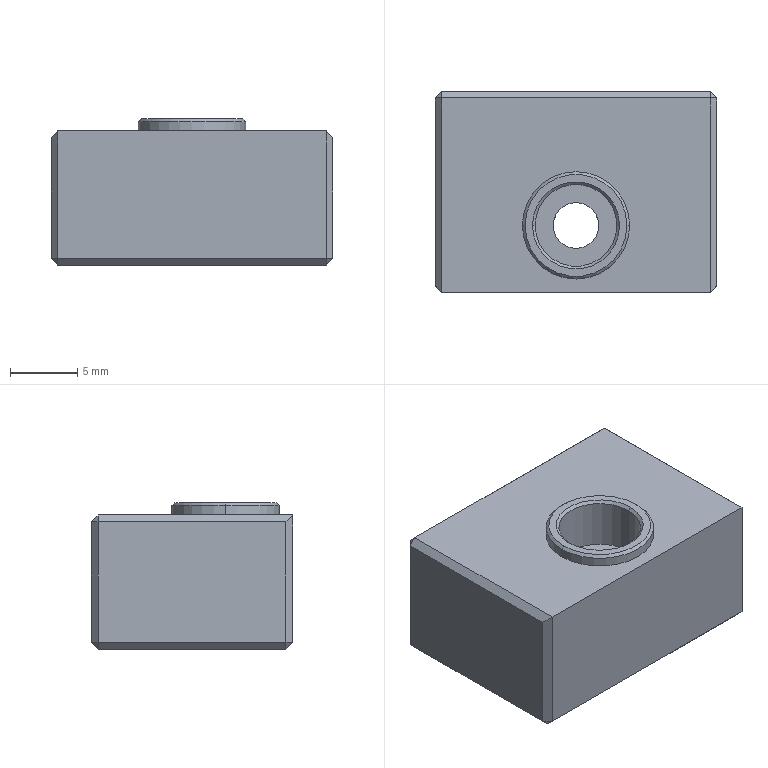Part | STEP file | 10000054265swp000-1 | 1 solid | 46 faces | box 21 x 15 x 10.9 mm | volume 2839 mm3 | plane 26 | cylinder 12 | cone 8 | commonest cylinder face diameters 2.5 x4 3.4 x2 6.1 x2 6.5 x2 8 x2
STEP:
#1=CARTESIAN_POINT('',(3.8,-2.5,5.9));
#2=VERTEX_POINT('',#1);
#3=CARTESIAN_POINT('',(-3.8,-2.5,5.9));
#4=VERTEX_POINT('',#3);
#5=CARTESIAN_POINT('',(0.,-2.5,5.9));
#6=DIRECTION('',(0.,0.,1.));
#7=DIRECTION('',(1.,0.,0.));
#8=AXIS2_PLACEMENT_3D('',#5,#6,#7);
#9=CIRCLE('',#8,3.8);
#10=EDGE_CURVE('',#2,#4,#9,.T.);
#11=ORIENTED_EDGE('',*,*,#10,.F.);
#12=CARTESIAN_POINT('',(4.,-2.5,5.7));
#13=VERTEX_POINT('',#12);
#14=CARTESIAN_POINT('',(3.8,-2.5,5.9));
#15=DIRECTION('',(0.7071,0.,-0.7071));
#16=VECTOR('',#15,1000.);
#17=LINE('',#14,#16);
#18=EDGE_CURVE('',#2,#13,#17,.T.);
#19=ORIENTED_EDGE('',*,*,#18,.T.);
#20=CARTESIAN_POINT('',(-4.,-2.5,5.7));
#21=VERTEX_POINT('',#20);
#22=CARTESIAN_POINT('',(0.,-2.5,5.7));
#23=DIRECTION('',(0.,0.,-1.));
#24=DIRECTION('',(1.,0.,0.));
#25=AXIS2_PLACEMENT_3D('',#22,#23,#24);
#26=CIRCLE('',#25,4.);
#27=EDGE_CURVE('',#21,#13,#26,.T.);
#28=ORIENTED_EDGE('',*,*,#27,.F.);
#29=CARTESIAN_POINT('',(-3.8,-2.5,5.9));
#30=DIRECTION('',(-0.7071,0.,-0.7071));
#31=VECTOR('',#30,1000.);
#32=LINE('',#29,#31);
#33=EDGE_CURVE('',#4,#21,#32,.T.);
#34=ORIENTED_EDGE('',*,*,#33,.F.);
#35=EDGE_LOOP('',(#11,#19,#28,#34));
#36=FACE_OUTER_BOUND('',#35,.T.);
#37=CARTESIAN_POINT('',(0.,-2.5,5.9));
#38=DIRECTION('',(0.,0.,-1.));
#39=DIRECTION('',(-1.,0.,0.));
#40=AXIS2_PLACEMENT_3D('',#37,#38,#39);
#41=CONICAL_SURFACE('',#40,3.8,0.7854);
#42=ADVANCED_FACE('',(#36),#41,.T.);
#43=CARTESIAN_POINT('',(-3.05,-2.5,5.7));
#44=VERTEX_POINT('',#43);
#45=CARTESIAN_POINT('',(3.05,-2.5,5.7));
#46=VERTEX_POINT('',#45);
#47=CARTESIAN_POINT('',(0.,-2.5,5.7));
#48=DIRECTION('',(0.,0.,1.));
#49=DIRECTION('',(1.,0.,0.));
#50=AXIS2_PLACEMENT_3D('',#47,#48,#49);
#51=CIRCLE('',#50,3.05);
#52=EDGE_CURVE('',#44,#46,#51,.T.);
#53=ORIENTED_EDGE('',*,*,#52,.F.);
#54=CARTESIAN_POINT('',(-3.25,-2.5,5.9));
#55=VERTEX_POINT('',#54);
#56=CARTESIAN_POINT('',(-3.05,-2.5,5.7));
#57=DIRECTION('',(-0.7071,0.,0.7071));
#58=VECTOR('',#57,1000.);
#59=LINE('',#56,#58);
#60=EDGE_CURVE('',#44,#55,#59,.T.);
#61=ORIENTED_EDGE('',*,*,#60,.T.);
#62=CARTESIAN_POINT('',(3.25,-2.5,5.9));
#63=VERTEX_POINT('',#62);
#64=CARTESIAN_POINT('',(0.,-2.5,5.9));
#65=DIRECTION('',(0.,0.,-1.));
#66=DIRECTION('',(1.,0.,0.));
#67=AXIS2_PLACEMENT_3D('',#64,#65,#66);
#68=CIRCLE('',#67,3.25);
#69=EDGE_CURVE('',#63,#55,#68,.T.);
#70=ORIENTED_EDGE('',*,*,#69,.F.);
#71=CARTESIAN_POINT('',(3.05,-2.5,5.7));
#72=DIRECTION('',(0.7071,0.,0.7071));
#73=VECTOR('',#72,1000.);
#74=LINE('',#71,#73);
#75=EDGE_CURVE('',#46,#63,#74,.T.);
#76=ORIENTED_EDGE('',*,*,#75,.F.);
#77=EDGE_LOOP('',(#53,#61,#70,#76));
#78=FACE_OUTER_BOUND('',#77,.T.);
#79=CARTESIAN_POINT('',(0.,-2.5,5.7));
#80=DIRECTION('',(0.,0.,1.));
#81=DIRECTION('',(1.,0.,0.));
#82=AXIS2_PLACEMENT_3D('',#79,#80,#81);
#83=CONICAL_SURFACE('',#82,3.05,0.7854);
#84=ADVANCED_FACE('',(#78),#83,.F.);
#85=CARTESIAN_POINT('',(3.25,-2.5,-1.6));
#86=VERTEX_POINT('',#85);
#87=CARTESIAN_POINT('',(-3.25,-2.5,-1.6));
#88=VERTEX_POINT('',#87);
#89=CARTESIAN_POINT('',(0.,-2.5,-1.6));
#90=DIRECTION('',(0.,0.,-1.));
#91=DIRECTION('',(-1.,0.,0.));
#92=AXIS2_PLACEMENT_3D('',#89,#90,#91);
#93=CIRCLE('',#92,3.25);
#94=EDGE_CURVE('',#86,#88,#93,.T.);
#95=ORIENTED_EDGE('',*,*,#94,.F.);
#96=CARTESIAN_POINT('',(3.25,-2.5,-5.));
#97=VERTEX_POINT('',#96);
#98=CARTESIAN_POINT('',(3.25,-2.5,-5.));
#99=DIRECTION('',(0.,0.,-1.));
#100=VECTOR('',#99,1000.);
#101=LINE('',#98,#100);
#102=EDGE_CURVE('',#86,#97,#101,.T.);
#103=ORIENTED_EDGE('',*,*,#102,.T.);
#104=CARTESIAN_POINT('',(-3.25,-2.5,-5.));
#105=VERTEX_POINT('',#104);
#106=CARTESIAN_POINT('',(0.,-2.5,-5.));
#107=DIRECTION('',(0.,0.,-1.));
#108=DIRECTION('',(-1.,0.,0.));
#109=AXIS2_PLACEMENT_3D('',#106,#107,#108);
#110=CIRCLE('',#109,3.25);
#111=EDGE_CURVE('',#97,#105,#110,.T.);
#112=ORIENTED_EDGE('',*,*,#111,.T.);
#113=CARTESIAN_POINT('',(-3.25,-2.5,-5.));
#114=DIRECTION('',(0.,0.,-1.));
#115=VECTOR('',#114,1000.);
#116=LINE('',#113,#115);
#117=EDGE_CURVE('',#88,#105,#116,.T.);
#118=ORIENTED_EDGE('',*,*,#117,.F.);
#119=EDGE_LOOP('',(#95,#103,#112,#118));
#120=FACE_OUTER_BOUND('',#119,.T.);
#121=CARTESIAN_POINT('',(0.,-2.5,-5.));
#122=DIRECTION('',(0.,0.,-1.));
#123=DIRECTION('',(-1.,0.,0.));
#124=AXIS2_PLACEMENT_3D('',#121,#122,#123);
#125=CYLINDRICAL_SURFACE('',#124,3.25);
#126=ADVANCED_FACE('',(#120),#125,.F.);
#127=CARTESIAN_POINT('',(1.7,-2.5,2.));
#128=VERTEX_POINT('',#127);
#129=CARTESIAN_POINT('',(-1.7,-2.5,2.));
#130=VERTEX_POINT('',#129);
#131=CARTESIAN_POINT('',(0.,-2.5,2.));
#132=DIRECTION('',(0.,0.,-1.));
#133=DIRECTION('',(-1.,0.,0.));
#134=AXIS2_PLACEMENT_3D('',#131,#132,#133);
#135=CIRCLE('',#134,1.7);
#136=EDGE_CURVE('',#128,#130,#135,.T.);
#137=ORIENTED_EDGE('',*,*,#136,.F.);
#138=CARTESIAN_POINT('',(1.7,-2.5,-1.6));
#139=VERTEX_POINT('',#138);
#140=CARTESIAN_POINT('',(1.7,-2.5,-5.));
#141=DIRECTION('',(0.,0.,-1.));
#142=VECTOR('',#141,1000.);
#143=LINE('',#140,#142);
#144=EDGE_CURVE('',#128,#139,#143,.T.);
#145=ORIENTED_EDGE('',*,*,#144,.T.);
#146=CARTESIAN_POINT('',(-1.7,-2.5,-1.6));
#147=VERTEX_POINT('',#146);
#148=CARTESIAN_POINT('',(0.,-2.5,-1.6));
#149=DIRECTION('',(0.,0.,-1.));
#150=DIRECTION('',(-1.,0.,0.));
#151=AXIS2_PLACEMENT_3D('',#148,#149,#150);
#152=CIRCLE('',#151,1.7);
#153=EDGE_CURVE('',#139,#147,#152,.T.);
#154=ORIENTED_EDGE('',*,*,#153,.T.);
#155=CARTESIAN_POINT('',(-1.7,-2.5,-5.));
#156=DIRECTION('',(0.,0.,-1.));
#157=VECTOR('',#156,1000.);
#158=LINE('',#155,#157);
#159=EDGE_CURVE('',#130,#147,#158,.T.);
#160=ORIENTED_EDGE('',*,*,#159,.F.);
#161=EDGE_LOOP('',(#137,#145,#154,#160));
#162=FACE_OUTER_BOUND('',#161,.T.);
#163=CARTESIAN_POINT('',(0.,-2.5,-5.));
#164=DIRECTION('',(0.,0.,-1.));
#165=DIRECTION('',(-1.,0.,0.));
#166=AXIS2_PLACEMENT_3D('',#163,#164,#165);
#167=CYLINDRICAL_SURFACE('',#166,1.7);
#168=ADVANCED_FACE('',(#162),#167,.F.);
#169=CARTESIAN_POINT('',(-3.05,-2.5,2.));
#170=VERTEX_POINT('',#169);
#171=CARTESIAN_POINT('',(3.05,-2.5,2.));
#172=VERTEX_POINT('',#171);
#173=CARTESIAN_POINT('',(0.,-2.5,2.));
#174=DIRECTION('',(0.,0.,1.));
#175=DIRECTION('',(1.,0.,0.));
#176=AXIS2_PLACEMENT_3D('',#173,#174,#175);
#177=CIRCLE('',#176,3.05);
#178=EDGE_CURVE('',#170,#172,#177,.T.);
#179=ORIENTED_EDGE('',*,*,#178,.F.);
#180=CARTESIAN_POINT('',(-3.05,-2.5,5.));
#181=DIRECTION('',(0.,0.,1.));
#182=VECTOR('',#181,1000.);
#183=LINE('',#180,#182);
#184=EDGE_CURVE('',#170,#44,#183,.T.);
#185=ORIENTED_EDGE('',*,*,#184,.T.);
#186=ORIENTED_EDGE('',*,*,#52,.T.);
#187=CARTESIAN_POINT('',(3.05,-2.5,5.));
#188=DIRECTION('',(0.,0.,1.));
#189=VECTOR('',#188,1000.);
#190=LINE('',#187,#189);
#191=EDGE_CURVE('',#172,#46,#190,.T.);
#192=ORIENTED_EDGE('',*,*,#191,.F.);
#193=EDGE_LOOP('',(#179,#185,#186,#192));
#194=FACE_OUTER_BOUND('',#193,.T.);
#195=CARTESIAN_POINT('',(0.,-2.5,5.));
#196=DIRECTION('',(0.,0.,1.));
#197=DIRECTION('',(1.,0.,0.));
#198=AXIS2_PLACEMENT_3D('',#195,#196,#197);
#199=CYLINDRICAL_SURFACE('',#198,3.05);
#200=ADVANCED_FACE('',(#194),#199,.F.);
#201=ORIENTED_EDGE('',*,*,#27,.T.);
#202=CARTESIAN_POINT('',(4.,-2.5,5.));
#203=VERTEX_POINT('',#202);
#204=CARTESIAN_POINT('',(4.,-2.5,5.9));
#205=DIRECTION('',(0.,0.,-1.));
#206=VECTOR('',#205,1000.);
#207=LINE('',#204,#206);
#208=EDGE_CURVE('',#13,#203,#207,.T.);
#209=ORIENTED_EDGE('',*,*,#208,.T.);
#210=CARTESIAN_POINT('',(-4.,-2.5,5.));
#211=VERTEX_POINT('',#210);
#212=CARTESIAN_POINT('',(0.,-2.5,5.));
#213=DIRECTION('',(0.,0.,1.));
#214=DIRECTION('',(1.,0.,0.));
#215=AXIS2_PLACEMENT_3D('',#212,#213,#214);
#216=CIRCLE('',#215,4.);
#217=EDGE_CURVE('',#203,#211,#216,.T.);
#218=ORIENTED_EDGE('',*,*,#217,.T.);
#219=CARTESIAN_POINT('',(-4.,-2.5,5.9));
#220=DIRECTION('',(0.,0.,-1.));
#221=VECTOR('',#220,1000.);
#222=LINE('',#219,#221);
#223=EDGE_CURVE('',#21,#211,#222,.T.);
#224=ORIENTED_EDGE('',*,*,#223,.F.);
#225=EDGE_LOOP('',(#201,#209,#218,#224));
#226=FACE_OUTER_BOUND('',#225,.T.);
#227=CARTESIAN_POINT('',(0.,-2.5,5.9));
#228=DIRECTION('',(0.,0.,-1.));
#229=DIRECTION('',(-1.,0.,0.));
#230=AXIS2_PLACEMENT_3D('',#227,#228,#229);
#231=CYLINDRICAL_SURFACE('',#230,4.);
#232=ADVANCED_FACE('',(#226),#231,.T.);
#233=CARTESIAN_POINT('',(-5.5,0.,-1.25));
#234=VERTEX_POINT('',#233);
#235=CARTESIAN_POINT('',(-5.5,0.,1.25));
#236=VERTEX_POINT('',#235);
#237=CARTESIAN_POINT('',(-5.5,0.,0.));
#238=DIRECTION('',(0.,1.,0.));
#239=DIRECTION('',(0.,0.,1.));
#240=AXIS2_PLACEMENT_3D('',#237,#238,#239);
#241=CIRCLE('',#240,1.25);
#242=EDGE_CURVE('',#234,#236,#241,.T.);
#243=ORIENTED_EDGE('',*,*,#242,.F.);
#244=CARTESIAN_POINT('',(-5.5,7.5,-1.25));
#245=VERTEX_POINT('',#244);
#246=CARTESIAN_POINT('',(-5.5,7.5,-1.25));
#247=DIRECTION('',(0.,1.,0.));
#248=VECTOR('',#247,1000.);
#249=LINE('',#246,#248);
#250=EDGE_CURVE('',#234,#245,#249,.T.);
#251=ORIENTED_EDGE('',*,*,#250,.T.);
#252=CARTESIAN_POINT('',(-5.5,7.5,1.25));
#253=VERTEX_POINT('',#252);
#254=CARTESIAN_POINT('',(-5.5,7.5,0.));
#255=DIRECTION('',(0.,1.,0.));
#256=DIRECTION('',(0.,0.,1.));
#257=AXIS2_PLACEMENT_3D('',#254,#255,#256);
#258=CIRCLE('',#257,1.25);
#259=EDGE_CURVE('',#245,#253,#258,.T.);
#260=ORIENTED_EDGE('',*,*,#259,.T.);
#261=CARTESIAN_POINT('',(-5.5,7.5,1.25));
#262=DIRECTION('',(0.,1.,0.));
#263=VECTOR('',#262,1000.);
#264=LINE('',#261,#263);
#265=EDGE_CURVE('',#236,#253,#264,.T.);
#266=ORIENTED_EDGE('',*,*,#265,.F.);
#267=EDGE_LOOP('',(#243,#251,#260,#266));
#268=FACE_OUTER_BOUND('',#267,.T.);
#269=CARTESIAN_POINT('',(-5.5,7.5,0.));
#270=DIRECTION('',(0.,1.,0.));
#271=DIRECTION('',(0.,0.,1.));
#272=AXIS2_PLACEMENT_3D('',#269,#270,#271);
#273=CYLINDRICAL_SURFACE('',#272,1.25);
#274=ADVANCED_FACE('',(#268),#273,.F.);
#275=CARTESIAN_POINT('',(-5.5,-0.7511,0.));
#276=VERTEX_POINT('',#275);
#277=CARTESIAN_POINT('',(-5.5,0.,1.25));
#278=DIRECTION('',(0.,0.515,0.8572));
#279=VECTOR('',#278,1000.);
#280=LINE('',#277,#279);
#281=EDGE_CURVE('',#276,#236,#280,.T.);
#282=ORIENTED_EDGE('',*,*,#281,.F.);
#283=CARTESIAN_POINT('',(-5.5,0.,-1.25));
#284=DIRECTION('',(0.,0.515,-0.8572));
#285=VECTOR('',#284,1000.);
#286=LINE('',#283,#285);
#287=EDGE_CURVE('',#276,#234,#286,.T.);
#288=ORIENTED_EDGE('',*,*,#287,.T.);
#289=ORIENTED_EDGE('',*,*,#242,.T.);
#290=EDGE_LOOP('',(#282,#288,#289));
#291=FACE_OUTER_BOUND('',#290,.T.);
#292=CARTESIAN_POINT('',(-5.5,0.,0.));
#293=DIRECTION('',(0.,1.,0.));
#294=DIRECTION('',(0.,0.,1.));
#295=AXIS2_PLACEMENT_3D('',#292,#293,#294);
#296=CONICAL_SURFACE('',#295,1.25,1.03);
#297=ADVANCED_FACE('',(#291),#296,.F.);
#298=CARTESIAN_POINT('',(5.5,0.,-1.25));
#299=VERTEX_POINT('',#298);
#300=CARTESIAN_POINT('',(5.5,0.,1.25));
#301=VERTEX_POINT('',#300);
#302=CARTESIAN_POINT('',(5.5,0.,0.));
#303=DIRECTION('',(0.,1.,0.));
#304=DIRECTION('',(0.,0.,1.));
#305=AXIS2_PLACEMENT_3D('',#302,#303,#304);
#306=CIRCLE('',#305,1.25);
#307=EDGE_CURVE('',#299,#301,#306,.T.);
#308=ORIENTED_EDGE('',*,*,#307,.F.);
#309=CARTESIAN_POINT('',(5.5,7.5,-1.25));
#310=VERTEX_POINT('',#309);
#311=CARTESIAN_POINT('',(5.5,7.5,-1.25));
#312=DIRECTION('',(0.,1.,0.));
#313=VECTOR('',#312,1000.);
#314=LINE('',#311,#313);
#315=EDGE_CURVE('',#299,#310,#314,.T.);
#316=ORIENTED_EDGE('',*,*,#315,.T.);
#317=CARTESIAN_POINT('',(5.5,7.5,1.25));
#318=VERTEX_POINT('',#317);
#319=CARTESIAN_POINT('',(5.5,7.5,0.));
#320=DIRECTION('',(0.,1.,0.));
#321=DIRECTION('',(0.,0.,1.));
#322=AXIS2_PLACEMENT_3D('',#319,#320,#321);
#323=CIRCLE('',#322,1.25);
#324=EDGE_CURVE('',#310,#318,#323,.T.);
#325=ORIENTED_EDGE('',*,*,#324,.T.);
#326=CARTESIAN_POINT('',(5.5,7.5,1.25));
#327=DIRECTION('',(0.,1.,0.));
#328=VECTOR('',#327,1000.);
#329=LINE('',#326,#328);
#330=EDGE_CURVE('',#301,#318,#329,.T.);
#331=ORIENTED_EDGE('',*,*,#330,.F.);
#332=EDGE_LOOP('',(#308,#316,#325,#331));
#333=FACE_OUTER_BOUND('',#332,.T.);
#334=CARTESIAN_POINT('',(5.5,7.5,0.));
#335=DIRECTION('',(0.,1.,0.));
#336=DIRECTION('',(0.,0.,1.));
#337=AXIS2_PLACEMENT_3D('',#334,#335,#336);
#338=CYLINDRICAL_SURFACE('',#337,1.25);
#339=ADVANCED_FACE('',(#333),#338,.F.);
#340=CARTESIAN_POINT('',(5.5,-0.7511,0.));
#341=VERTEX_POINT('',#340);
#342=CARTESIAN_POINT('',(5.5,0.,1.25));
#343=DIRECTION('',(0.,0.515,0.8572));
#344=VECTOR('',#343,1000.);
#345=LINE('',#342,#344);
#346=EDGE_CURVE('',#341,#301,#345,.T.);
#347=ORIENTED_EDGE('',*,*,#346,.F.);
#348=CARTESIAN_POINT('',(5.5,0.,-1.25));
#349=DIRECTION('',(0.,0.515,-0.8572));
#350=VECTOR('',#349,1000.);
#351=LINE('',#348,#350);
#352=EDGE_CURVE('',#341,#299,#351,.T.);
#353=ORIENTED_EDGE('',*,*,#352,.T.);
#354=ORIENTED_EDGE('',*,*,#307,.T.);
#355=EDGE_LOOP('',(#347,#353,#354));
#356=FACE_OUTER_BOUND('',#355,.T.);
#357=CARTESIAN_POINT('',(5.5,0.,0.));
#358=DIRECTION('',(0.,1.,0.));
#359=DIRECTION('',(0.,0.,1.));
#360=AXIS2_PLACEMENT_3D('',#357,#358,#359);
#361=CONICAL_SURFACE('',#360,1.25,1.03);
#362=ADVANCED_FACE('',(#356),#361,.F.);
#363=CARTESIAN_POINT('',(-10.,-7.5,5.));
#364=VERTEX_POINT('',#363);
#365=CARTESIAN_POINT('',(10.,-7.5,5.));
#366=VERTEX_POINT('',#365);
#367=CARTESIAN_POINT('',(-10.5,-7.5,5.));
#368=DIRECTION('',(1.,0.,0.));
#369=VECTOR('',#368,1000.);
#370=LINE('',#367,#369);
#371=EDGE_CURVE('',#364,#366,#370,.T.);
#372=ORIENTED_EDGE('',*,*,#371,.T.);
#373=CARTESIAN_POINT('',(10.,7.,5.));
#374=VERTEX_POINT('',#373);
#375=CARTESIAN_POINT('',(10.,7.5,5.));
#376=DIRECTION('',(0.,1.,0.));
#377=VECTOR('',#376,1000.);
#378=LINE('',#375,#377);
#379=EDGE_CURVE('',#366,#374,#378,.T.);
#380=ORIENTED_EDGE('',*,*,#379,.T.);
#381=CARTESIAN_POINT('',(-10.,7.,5.));
#382=VERTEX_POINT('',#381);
#383=CARTESIAN_POINT('',(-10.5,7.,5.));
#384=DIRECTION('',(-1.,0.,0.));
#385=VECTOR('',#384,1000.);
#386=LINE('',#383,#385);
#387=EDGE_CURVE('',#374,#382,#386,.T.);
#388=ORIENTED_EDGE('',*,*,#387,.T.);
#389=CARTESIAN_POINT('',(-10.,-7.5,5.));
#390=DIRECTION('',(0.,-1.,0.));
#391=VECTOR('',#390,1000.);
#392=LINE('',#389,#391);
#393=EDGE_CURVE('',#382,#364,#392,.T.);
#394=ORIENTED_EDGE('',*,*,#393,.T.);
#395=EDGE_LOOP('',(#372,#380,#388,#394));
#396=FACE_OUTER_BOUND('',#395,.T.);
#397=CARTESIAN_POINT('',(0.,-2.5,5.));
#398=DIRECTION('',(0.,0.,1.));
#399=DIRECTION('',(1.,0.,0.));
#400=AXIS2_PLACEMENT_3D('',#397,#398,#399);
#401=CIRCLE('',#400,4.);
#402=EDGE_CURVE('',#211,#203,#401,.T.);
#403=ORIENTED_EDGE('',*,*,#402,.F.);
#404=ORIENTED_EDGE('',*,*,#217,.F.);
#405=EDGE_LOOP('',(#403,#404));
#406=FACE_BOUND('',#405,.T.);
#407=CARTESIAN_POINT('',(0.,0.,5.));
#408=DIRECTION('',(0.,0.,1.));
#409=DIRECTION('',(1.,0.,0.));
#410=AXIS2_PLACEMENT_3D('',#407,#408,#409);
#411=PLANE('',#410);
#412=ADVANCED_FACE('',(#396,#406),#411,.T.);
#413=CARTESIAN_POINT('',(10.5,7.,-4.5));
#414=VERTEX_POINT('',#413);
#415=CARTESIAN_POINT('',(10.5,7.,4.5));
#416=VERTEX_POINT('',#415);
#417=CARTESIAN_POINT('',(10.5,7.,5.));
#418=DIRECTION('',(0.,0.,1.));
#419=VECTOR('',#418,1000.);
#420=LINE('',#417,#419);
#421=EDGE_CURVE('',#414,#416,#420,.T.);
#422=ORIENTED_EDGE('',*,*,#421,.T.);
#423=CARTESIAN_POINT('',(10.5,-7.,4.5));
#424=VERTEX_POINT('',#423);
#425=CARTESIAN_POINT('',(10.5,-7.5,4.5));
#426=DIRECTION('',(0.,-1.,0.));
#427=VECTOR('',#426,1000.);
#428=LINE('',#425,#427);
#429=EDGE_CURVE('',#416,#424,#428,.T.);
#430=ORIENTED_EDGE('',*,*,#429,.T.);
#431=CARTESIAN_POINT('',(10.5,-7.,-4.5));
#432=VERTEX_POINT('',#431);
#433=CARTESIAN_POINT('',(10.5,-7.,5.));
#434=DIRECTION('',(0.,0.,-1.));
#435=VECTOR('',#434,1000.);
#436=LINE('',#433,#435);
#437=EDGE_CURVE('',#424,#432,#436,.T.);
#438=ORIENTED_EDGE('',*,*,#437,.T.);
#439=CARTESIAN_POINT('',(10.5,7.5,-4.5));
#440=DIRECTION('',(0.,1.,0.));
#441=VECTOR('',#440,1000.);
#442=LINE('',#439,#441);
#443=EDGE_CURVE('',#432,#414,#442,.T.);
#444=ORIENTED_EDGE('',*,*,#443,.T.);
#445=EDGE_LOOP('',(#422,#430,#438,#444));
#446=FACE_OUTER_BOUND('',#445,.T.);
#447=CARTESIAN_POINT('',(10.5,7.5,5.));
#448=DIRECTION('',(-1.,0.,0.));
#449=DIRECTION('',(0.,0.,1.));
#450=AXIS2_PLACEMENT_3D('',#447,#448,#449);
#451=PLANE('',#450);
#452=ADVANCED_FACE('',(#446),#451,.F.);
#453=CARTESIAN_POINT('',(-10.,7.5,-4.5));
#454=VERTEX_POINT('',#453);
#455=CARTESIAN_POINT('',(-10.,7.5,4.5));
#456=VERTEX_POINT('',#455);
#457=CARTESIAN_POINT('',(-10.,7.5,5.));
#458=DIRECTION('',(0.,0.,1.));
#459=VECTOR('',#458,1000.);
#460=LINE('',#457,#459);
#461=EDGE_CURVE('',#454,#456,#460,.T.);
#462=ORIENTED_EDGE('',*,*,#461,.T.);
#463=CARTESIAN_POINT('',(10.,7.5,4.5));
#464=VERTEX_POINT('',#463);
#465=CARTESIAN_POINT('',(10.5,7.5,4.5));
#466=DIRECTION('',(1.,0.,0.));
#467=VECTOR('',#466,1000.);
#468=LINE('',#465,#467);
#469=EDGE_CURVE('',#456,#464,#468,.T.);
#470=ORIENTED_EDGE('',*,*,#469,.T.);
#471=CARTESIAN_POINT('',(10.,7.5,-4.5));
#472=VERTEX_POINT('',#471);
#473=CARTESIAN_POINT('',(10.,7.5,5.));
#474=DIRECTION('',(0.,0.,-1.));
#475=VECTOR('',#474,1000.);
#476=LINE('',#473,#475);
#477=EDGE_CURVE('',#464,#472,#476,.T.);
#478=ORIENTED_EDGE('',*,*,#477,.T.);
#479=CARTESIAN_POINT('',(-10.5,7.5,-4.5));
#480=DIRECTION('',(-1.,0.,0.));
#481=VECTOR('',#480,1000.);
#482=LINE('',#479,#481);
#483=EDGE_CURVE('',#472,#454,#482,.T.);
#484=ORIENTED_EDGE('',*,*,#483,.T.);
#485=EDGE_LOOP('',(#462,#470,#478,#484));
#486=FACE_OUTER_BOUND('',#485,.T.);
#487=CARTESIAN_POINT('',(-5.5,7.5,0.));
#488=DIRECTION('',(0.,1.,0.));
#489=DIRECTION('',(0.,0.,1.));
#490=AXIS2_PLACEMENT_3D('',#487,#488,#489);
#491=CIRCLE('',#490,1.25);
#492=EDGE_CURVE('',#253,#245,#491,.T.);
#493=ORIENTED_EDGE('',*,*,#492,.F.);
#494=ORIENTED_EDGE('',*,*,#259,.F.);
#495=EDGE_LOOP('',(#493,#494));
#496=FACE_BOUND('',#495,.T.);
#497=CARTESIAN_POINT('',(5.5,7.5,0.));
#498=DIRECTION('',(0.,1.,0.));
#499=DIRECTION('',(0.,0.,1.));
#500=AXIS2_PLACEMENT_3D('',#497,#498,#499);
#501=CIRCLE('',#500,1.25);
#502=EDGE_CURVE('',#318,#310,#501,.T.);
#503=ORIENTED_EDGE('',*,*,#502,.F.);
#504=ORIENTED_EDGE('',*,*,#324,.F.);
#505=EDGE_LOOP('',(#503,#504));
#506=FACE_BOUND('',#505,.T.);
#507=CARTESIAN_POINT('',(-10.5,7.5,5.));
#508=DIRECTION('',(0.,-1.,0.));
#509=DIRECTION('',(0.,0.,-1.));
#510=AXIS2_PLACEMENT_3D('',#507,#508,#509);
#511=PLANE('',#510);
#512=ADVANCED_FACE('',(#486,#496,#506),#511,.F.);
#513=CARTESIAN_POINT('',(-10.5,-7.,-4.5));
#514=VERTEX_POINT('',#513);
#515=CARTESIAN_POINT('',(-10.5,-7.,4.5));
#516=VERTEX_POINT('',#515);
#517=CARTESIAN_POINT('',(-10.5,-7.,5.));
#518=DIRECTION('',(0.,0.,1.));
#519=VECTOR('',#518,1000.);
#520=LINE('',#517,#519);
#521=EDGE_CURVE('',#514,#516,#520,.T.);
#522=ORIENTED_EDGE('',*,*,#521,.T.);
#523=CARTESIAN_POINT('',(-10.5,7.,4.5));
#524=VERTEX_POINT('',#523);
#525=CARTESIAN_POINT('',(-10.5,7.5,4.5));
#526=DIRECTION('',(0.,1.,0.));
#527=VECTOR('',#526,1000.);
#528=LINE('',#525,#527);
#529=EDGE_CURVE('',#516,#524,#528,.T.);
#530=ORIENTED_EDGE('',*,*,#529,.T.);
#531=CARTESIAN_POINT('',(-10.5,7.,-4.5));
#532=VERTEX_POINT('',#531);
#533=CARTESIAN_POINT('',(-10.5,7.,5.));
#534=DIRECTION('',(0.,0.,-1.));
#535=VECTOR('',#534,1000.);
#536=LINE('',#533,#535);
#537=EDGE_CURVE('',#524,#532,#536,.T.);
#538=ORIENTED_EDGE('',*,*,#537,.T.);
#539=CARTESIAN_POINT('',(-10.5,7.5,-4.5));
#540=DIRECTION('',(0.,-1.,0.));
#541=VECTOR('',#540,1000.);
#542=LINE('',#539,#541);
#543=EDGE_CURVE('',#532,#514,#542,.T.);
#544=ORIENTED_EDGE('',*,*,#543,.T.);
#545=EDGE_LOOP('',(#522,#530,#538,#544));
#546=FACE_OUTER_BOUND('',#545,.T.);
#547=CARTESIAN_POINT('',(-10.5,7.5,5.));
#548=DIRECTION('',(1.,0.,0.));
#549=DIRECTION('',(0.,0.,-1.));
#550=AXIS2_PLACEMENT_3D('',#547,#548,#549);
#551=PLANE('',#550);
#552=ADVANCED_FACE('',(#546),#551,.F.);
#553=ORIENTED_EDGE('',*,*,#371,.F.);
#554=CARTESIAN_POINT('',(-10.,-7.5,-4.5));
#555=VERTEX_POINT('',#554);
#556=CARTESIAN_POINT('',(-10.,-7.5,5.));
#557=DIRECTION('',(0.,0.,-1.));
#558=VECTOR('',#557,1000.);
#559=LINE('',#556,#558);
#560=EDGE_CURVE('',#364,#555,#559,.T.);
#561=ORIENTED_EDGE('',*,*,#560,.T.);
#562=CARTESIAN_POINT('',(10.,-7.5,-4.5));
#563=VERTEX_POINT('',#562);
#564=CARTESIAN_POINT('',(-10.5,-7.5,-4.5));
#565=DIRECTION('',(1.,0.,0.));
#566=VECTOR('',#565,1000.);
#567=LINE('',#564,#566);
#568=EDGE_CURVE('',#555,#563,#567,.T.);
#569=ORIENTED_EDGE('',*,*,#568,.T.);
#570=CARTESIAN_POINT('',(10.,-7.5,5.));
#571=DIRECTION('',(0.,0.,1.));
#572=VECTOR('',#571,1000.);
#573=LINE('',#570,#572);
#574=EDGE_CURVE('',#563,#366,#573,.T.);
#575=ORIENTED_EDGE('',*,*,#574,.T.);
#576=EDGE_LOOP('',(#553,#561,#569,#575));
#577=FACE_OUTER_BOUND('',#576,.T.);
#578=CARTESIAN_POINT('',(-10.5,-7.5,5.));
#579=DIRECTION('',(0.,1.,0.));
#580=DIRECTION('',(0.,0.,1.));
#581=AXIS2_PLACEMENT_3D('',#578,#579,#580);
#582=PLANE('',#581);
#583=ADVANCED_FACE('',(#577),#582,.F.);
#584=CARTESIAN_POINT('',(10.,7.,-5.));
#585=VERTEX_POINT('',#584);
#586=CARTESIAN_POINT('',(10.,-7.,-5.));
#587=VERTEX_POINT('',#586);
#588=CARTESIAN_POINT('',(10.,0.,-5.));
#589=DIRECTION('',(0.,-1.,0.));
#590=VECTOR('',#589,1000.);
#591=LINE('',#588,#590);
#592=EDGE_CURVE('',#585,#587,#591,.T.);
#593=ORIENTED_EDGE('',*,*,#592,.T.);
#594=CARTESIAN_POINT('',(-10.,-7.,-5.));
#595=VERTEX_POINT('',#594);
#596=CARTESIAN_POINT('',(0.,-7.,-5.));
#597=DIRECTION('',(-1.,0.,0.));
#598=VECTOR('',#597,1000.);
#599=LINE('',#596,#598);
#600=EDGE_CURVE('',#587,#595,#599,.T.);
#601=ORIENTED_EDGE('',*,*,#600,.T.);
#602=CARTESIAN_POINT('',(-10.,7.,-5.));
#603=VERTEX_POINT('',#602);
#604=CARTESIAN_POINT('',(-10.,0.,-5.));
#605=DIRECTION('',(0.,1.,0.));
#606=VECTOR('',#605,1000.);
#607=LINE('',#604,#606);
#608=EDGE_CURVE('',#595,#603,#607,.T.);
#609=ORIENTED_EDGE('',*,*,#608,.T.);
#610=CARTESIAN_POINT('',(0.,7.,-5.));
#611=DIRECTION('',(1.,0.,0.));
#612=VECTOR('',#611,1000.);
#613=LINE('',#610,#612);
#614=EDGE_CURVE('',#603,#585,#613,.T.);
#615=ORIENTED_EDGE('',*,*,#614,.T.);
#616=EDGE_LOOP('',(#593,#601,#609,#615));
#617=FACE_OUTER_BOUND('',#616,.T.);
#618=CARTESIAN_POINT('',(0.,-2.5,-5.));
#619=DIRECTION('',(0.,0.,-1.));
#620=DIRECTION('',(-1.,0.,0.));
#621=AXIS2_PLACEMENT_3D('',#618,#619,#620);
#622=CIRCLE('',#621,3.25);
#623=EDGE_CURVE('',#105,#97,#622,.T.);
#624=ORIENTED_EDGE('',*,*,#623,.F.);
#625=ORIENTED_EDGE('',*,*,#111,.F.);
#626=EDGE_LOOP('',(#624,#625));
#627=FACE_BOUND('',#626,.T.);
#628=CARTESIAN_POINT('',(0.,0.,-5.));
#629=DIRECTION('',(0.,0.,1.));
#630=DIRECTION('',(1.,0.,0.));
#631=AXIS2_PLACEMENT_3D('',#628,#629,#630);
#632=PLANE('',#631);
#633=ADVANCED_FACE('',(#617,#627),#632,.F.);
#634=ORIENTED_EDGE('',*,*,#352,.F.);
#635=ORIENTED_EDGE('',*,*,#346,.T.);
#636=CARTESIAN_POINT('',(5.5,0.,0.));
#637=DIRECTION('',(0.,1.,0.));
#638=DIRECTION('',(0.,0.,1.));
#639=AXIS2_PLACEMENT_3D('',#636,#637,#638);
#640=CIRCLE('',#639,1.25);
#641=EDGE_CURVE('',#301,#299,#640,.T.);
#642=ORIENTED_EDGE('',*,*,#641,.T.);
#643=EDGE_LOOP('',(#634,#635,#642));
#644=FACE_OUTER_BOUND('',#643,.T.);
#645=CARTESIAN_POINT('',(5.5,0.,0.));
#646=DIRECTION('',(0.,1.,0.));
#647=DIRECTION('',(0.,0.,1.));
#648=AXIS2_PLACEMENT_3D('',#645,#646,#647);
#649=CONICAL_SURFACE('',#648,1.25,1.03);
#650=ADVANCED_FACE('',(#644),#649,.F.);
#651=ORIENTED_EDGE('',*,*,#315,.F.);
#652=ORIENTED_EDGE('',*,*,#641,.F.);
#653=ORIENTED_EDGE('',*,*,#330,.T.);
#654=ORIENTED_EDGE('',*,*,#502,.T.);
#655=EDGE_LOOP('',(#651,#652,#653,#654));
#656=FACE_OUTER_BOUND('',#655,.T.);
#657=CARTESIAN_POINT('',(5.5,7.5,0.));
#658=DIRECTION('',(0.,1.,0.));
#659=DIRECTION('',(0.,0.,1.));
#660=AXIS2_PLACEMENT_3D('',#657,#658,#659);
#661=CYLINDRICAL_SURFACE('',#660,1.25);
#662=ADVANCED_FACE('',(#656),#661,.F.);
#663=ORIENTED_EDGE('',*,*,#287,.F.);
#664=ORIENTED_EDGE('',*,*,#281,.T.);
#665=CARTESIAN_POINT('',(-5.5,0.,0.));
#666=DIRECTION('',(0.,1.,0.));
#667=DIRECTION('',(0.,0.,1.));
#668=AXIS2_PLACEMENT_3D('',#665,#666,#667);
#669=CIRCLE('',#668,1.25);
#670=EDGE_CURVE('',#236,#234,#669,.T.);
#671=ORIENTED_EDGE('',*,*,#670,.T.);
#672=EDGE_LOOP('',(#663,#664,#671));
#673=FACE_OUTER_BOUND('',#672,.T.);
#674=CARTESIAN_POINT('',(-5.5,0.,0.));
#675=DIRECTION('',(0.,1.,0.));
#676=DIRECTION('',(0.,0.,1.));
#677=AXIS2_PLACEMENT_3D('',#674,#675,#676);
#678=CONICAL_SURFACE('',#677,1.25,1.03);
#679=ADVANCED_FACE('',(#673),#678,.F.);
#680=ORIENTED_EDGE('',*,*,#250,.F.);
#681=ORIENTED_EDGE('',*,*,#670,.F.);
#682=ORIENTED_EDGE('',*,*,#265,.T.);
#683=ORIENTED_EDGE('',*,*,#492,.T.);
#684=EDGE_LOOP('',(#680,#681,#682,#683));
#685=FACE_OUTER_BOUND('',#684,.T.);
#686=CARTESIAN_POINT('',(-5.5,7.5,0.));
#687=DIRECTION('',(0.,1.,0.));
#688=DIRECTION('',(0.,0.,1.));
#689=AXIS2_PLACEMENT_3D('',#686,#687,#688);
#690=CYLINDRICAL_SURFACE('',#689,1.25);
#691=ADVANCED_FACE('',(#685),#690,.F.);
#692=ORIENTED_EDGE('',*,*,#69,.T.);
#693=CARTESIAN_POINT('',(0.,-2.5,5.9));
#694=DIRECTION('',(0.,0.,-1.));
#695=DIRECTION('',(1.,0.,0.));
#696=AXIS2_PLACEMENT_3D('',#693,#694,#695);
#697=CIRCLE('',#696,3.25);
#698=EDGE_CURVE('',#55,#63,#697,.T.);
#699=ORIENTED_EDGE('',*,*,#698,.T.);
#700=EDGE_LOOP('',(#692,#699));
#701=FACE_BOUND('',#700,.T.);
#702=CARTESIAN_POINT('',(0.,-2.5,5.9));
#703=DIRECTION('',(0.,0.,1.));
#704=DIRECTION('',(1.,0.,0.));
#705=AXIS2_PLACEMENT_3D('',#702,#703,#704);
#706=CIRCLE('',#705,3.8);
#707=EDGE_CURVE('',#4,#2,#706,.T.);
#708=ORIENTED_EDGE('',*,*,#707,.T.);
#709=ORIENTED_EDGE('',*,*,#10,.T.);
#710=EDGE_LOOP('',(#708,#709));
#711=FACE_OUTER_BOUND('',#710,.T.);
#712=CARTESIAN_POINT('',(0.,-2.5,5.9));
#713=DIRECTION('',(0.,0.,1.));
#714=DIRECTION('',(1.,0.,0.));
#715=AXIS2_PLACEMENT_3D('',#712,#713,#714);
#716=PLANE('',#715);
#717=ADVANCED_FACE('',(#701,#711),#716,.T.);
#718=ORIENTED_EDGE('',*,*,#208,.F.);
#719=CARTESIAN_POINT('',(0.,-2.5,5.7));
#720=DIRECTION('',(0.,0.,-1.));
#721=DIRECTION('',(1.,0.,0.));
#722=AXIS2_PLACEMENT_3D('',#719,#720,#721);
#723=CIRCLE('',#722,4.);
#724=EDGE_CURVE('',#13,#21,#723,.T.);
#725=ORIENTED_EDGE('',*,*,#724,.T.);
#726=ORIENTED_EDGE('',*,*,#223,.T.);
#727=ORIENTED_EDGE('',*,*,#402,.T.);
#728=EDGE_LOOP('',(#718,#725,#726,#727));
#729=FACE_OUTER_BOUND('',#728,.T.);
#730=CARTESIAN_POINT('',(0.,-2.5,5.9));
#731=DIRECTION('',(0.,0.,-1.));
#732=DIRECTION('',(-1.,0.,0.));
#733=AXIS2_PLACEMENT_3D('',#730,#731,#732);
#734=CYLINDRICAL_SURFACE('',#733,4.);
#735=ADVANCED_FACE('',(#729),#734,.T.);
#736=CARTESIAN_POINT('',(0.,-2.5,2.));
#737=DIRECTION('',(0.,0.,-1.));
#738=DIRECTION('',(-1.,0.,0.));
#739=AXIS2_PLACEMENT_3D('',#736,#737,#738);
#740=CIRCLE('',#739,1.7);
#741=EDGE_CURVE('',#130,#128,#740,.T.);
#742=ORIENTED_EDGE('',*,*,#741,.T.);
#743=ORIENTED_EDGE('',*,*,#136,.T.);
#744=EDGE_LOOP('',(#742,#743));
#745=FACE_BOUND('',#744,.T.);
#746=CARTESIAN_POINT('',(0.,-2.5,2.));
#747=DIRECTION('',(0.,0.,1.));
#748=DIRECTION('',(1.,0.,0.));
#749=AXIS2_PLACEMENT_3D('',#746,#747,#748);
#750=CIRCLE('',#749,3.05);
#751=EDGE_CURVE('',#172,#170,#750,.T.);
#752=ORIENTED_EDGE('',*,*,#751,.T.);
#753=ORIENTED_EDGE('',*,*,#178,.T.);
#754=EDGE_LOOP('',(#752,#753));
#755=FACE_OUTER_BOUND('',#754,.T.);
#756=CARTESIAN_POINT('',(0.,-2.5,2.));
#757=DIRECTION('',(0.,0.,-1.));
#758=DIRECTION('',(-1.,0.,0.));
#759=AXIS2_PLACEMENT_3D('',#756,#757,#758);
#760=PLANE('',#759);
#761=ADVANCED_FACE('',(#745,#755),#760,.F.);
#762=ORIENTED_EDGE('',*,*,#184,.F.);
#763=ORIENTED_EDGE('',*,*,#751,.F.);
#764=ORIENTED_EDGE('',*,*,#191,.T.);
#765=CARTESIAN_POINT('',(0.,-2.5,5.7));
#766=DIRECTION('',(0.,0.,1.));
#767=DIRECTION('',(1.,0.,0.));
#768=AXIS2_PLACEMENT_3D('',#765,#766,#767);
#769=CIRCLE('',#768,3.05);
#770=EDGE_CURVE('',#46,#44,#769,.T.);
#771=ORIENTED_EDGE('',*,*,#770,.T.);
#772=EDGE_LOOP('',(#762,#763,#764,#771));
#773=FACE_OUTER_BOUND('',#772,.T.);
#774=CARTESIAN_POINT('',(0.,-2.5,5.));
#775=DIRECTION('',(0.,0.,1.));
#776=DIRECTION('',(1.,0.,0.));
#777=AXIS2_PLACEMENT_3D('',#774,#775,#776);
#778=CYLINDRICAL_SURFACE('',#777,3.05);
#779=ADVANCED_FACE('',(#773),#778,.F.);
#780=ORIENTED_EDGE('',*,*,#144,.F.);
#781=ORIENTED_EDGE('',*,*,#741,.F.);
#782=ORIENTED_EDGE('',*,*,#159,.T.);
#783=CARTESIAN_POINT('',(0.,-2.5,-1.6));
#784=DIRECTION('',(0.,0.,-1.));
#785=DIRECTION('',(-1.,0.,0.));
#786=AXIS2_PLACEMENT_3D('',#783,#784,#785);
#787=CIRCLE('',#786,1.7);
#788=EDGE_CURVE('',#147,#139,#787,.T.);
#789=ORIENTED_EDGE('',*,*,#788,.T.);
#790=EDGE_LOOP('',(#780,#781,#782,#789));
#791=FACE_OUTER_BOUND('',#790,.T.);
#792=CARTESIAN_POINT('',(0.,-2.5,-5.));
#793=DIRECTION('',(0.,0.,-1.));
#794=DIRECTION('',(-1.,0.,0.));
#795=AXIS2_PLACEMENT_3D('',#792,#793,#794);
#796=CYLINDRICAL_SURFACE('',#795,1.7);
#797=ADVANCED_FACE('',(#791),#796,.F.);
#798=ORIENTED_EDGE('',*,*,#788,.F.);
#799=ORIENTED_EDGE('',*,*,#153,.F.);
#800=EDGE_LOOP('',(#798,#799));
#801=FACE_BOUND('',#800,.T.);
#802=CARTESIAN_POINT('',(0.,-2.5,-1.6));
#803=DIRECTION('',(0.,0.,-1.));
#804=DIRECTION('',(-1.,0.,0.));
#805=AXIS2_PLACEMENT_3D('',#802,#803,#804);
#806=CIRCLE('',#805,3.25);
#807=EDGE_CURVE('',#88,#86,#806,.T.);
#808=ORIENTED_EDGE('',*,*,#807,.T.);
#809=ORIENTED_EDGE('',*,*,#94,.T.);
#810=EDGE_LOOP('',(#808,#809));
#811=FACE_OUTER_BOUND('',#810,.T.);
#812=CARTESIAN_POINT('',(1.7,-2.5,-1.6));
#813=DIRECTION('',(0.,0.,1.));
#814=DIRECTION('',(1.,0.,0.));
#815=AXIS2_PLACEMENT_3D('',#812,#813,#814);
#816=PLANE('',#815);
#817=ADVANCED_FACE('',(#801,#811),#816,.F.);
#818=ORIENTED_EDGE('',*,*,#102,.F.);
#819=ORIENTED_EDGE('',*,*,#807,.F.);
#820=ORIENTED_EDGE('',*,*,#117,.T.);
#821=ORIENTED_EDGE('',*,*,#623,.T.);
#822=EDGE_LOOP('',(#818,#819,#820,#821));
#823=FACE_OUTER_BOUND('',#822,.T.);
#824=CARTESIAN_POINT('',(0.,-2.5,-5.));
#825=DIRECTION('',(0.,0.,-1.));
#826=DIRECTION('',(-1.,0.,0.));
#827=AXIS2_PLACEMENT_3D('',#824,#825,#826);
#828=CYLINDRICAL_SURFACE('',#827,3.25);
#829=ADVANCED_FACE('',(#823),#828,.F.);
#830=CARTESIAN_POINT('',(-10.,-7.,-5.));
#831=DIRECTION('',(0.7071,0.,-0.7071));
#832=VECTOR('',#831,1000.);
#833=LINE('',#830,#832);
#834=EDGE_CURVE('',#514,#595,#833,.T.);
#835=ORIENTED_EDGE('',*,*,#834,.F.);
#836=ORIENTED_EDGE('',*,*,#543,.F.);
#837=CARTESIAN_POINT('',(-10.,7.,-5.));
#838=DIRECTION('',(-0.7071,0.,0.7071));
#839=VECTOR('',#838,1000.);
#840=LINE('',#837,#839);
#841=EDGE_CURVE('',#603,#532,#840,.T.);
#842=ORIENTED_EDGE('',*,*,#841,.F.);
#843=ORIENTED_EDGE('',*,*,#608,.F.);
#844=EDGE_LOOP('',(#835,#836,#842,#843));
#845=FACE_OUTER_BOUND('',#844,.T.);
#846=CARTESIAN_POINT('',(-10.5,7.5,-4.5));
#847=DIRECTION('',(0.7071,0.,0.7071));
#848=DIRECTION('',(0.,-1.,0.));
#849=AXIS2_PLACEMENT_3D('',#846,#847,#848);
#850=PLANE('',#849);
#851=ADVANCED_FACE('',(#845),#850,.F.);
#852=CARTESIAN_POINT('',(-10.,-7.5,5.));
#853=DIRECTION('',(0.5774,-0.5774,0.5774));
#854=VECTOR('',#853,1000.);
#855=LINE('',#852,#854);
#856=EDGE_CURVE('',#516,#364,#855,.T.);
#857=ORIENTED_EDGE('',*,*,#856,.F.);
#858=ORIENTED_EDGE('',*,*,#521,.F.);
#859=CARTESIAN_POINT('',(-10.25,-7.25,-4.5));
#860=DIRECTION('',(-0.7071,0.7071,0.));
#861=VECTOR('',#860,1000.);
#862=LINE('',#859,#861);
#863=EDGE_CURVE('',#555,#514,#862,.T.);
#864=ORIENTED_EDGE('',*,*,#863,.F.);
#865=ORIENTED_EDGE('',*,*,#560,.F.);
#866=EDGE_LOOP('',(#857,#858,#864,#865));
#867=FACE_OUTER_BOUND('',#866,.T.);
#868=CARTESIAN_POINT('',(-10.,-7.5,5.));
#869=DIRECTION('',(0.7071,0.7071,0.));
#870=DIRECTION('',(0.,0.,-1.));
#871=AXIS2_PLACEMENT_3D('',#868,#869,#870);
#872=PLANE('',#871);
#873=ADVANCED_FACE('',(#867),#872,.F.);
#874=CARTESIAN_POINT('',(-10.,7.,-5.));
#875=DIRECTION('',(0.,0.7071,0.7071));
#876=VECTOR('',#875,1000.);
#877=LINE('',#874,#876);
#878=EDGE_CURVE('',#603,#454,#877,.T.);
#879=ORIENTED_EDGE('',*,*,#878,.F.);
#880=ORIENTED_EDGE('',*,*,#841,.T.);
#881=CARTESIAN_POINT('',(-10.25,7.25,-4.5));
#882=DIRECTION('',(-0.7071,-0.7071,0.));
#883=VECTOR('',#882,1000.);
#884=LINE('',#881,#883);
#885=EDGE_CURVE('',#454,#532,#884,.T.);
#886=ORIENTED_EDGE('',*,*,#885,.F.);
#887=EDGE_LOOP('',(#879,#880,#886));
#888=FACE_OUTER_BOUND('',#887,.T.);
#889=CARTESIAN_POINT('',(-10.,7.,-5.));
#890=DIRECTION('',(-0.5774,0.5774,-0.5774));
#891=DIRECTION('',(-0.7071,0.,0.7071));
#892=AXIS2_PLACEMENT_3D('',#889,#890,#891);
#893=PLANE('',#892);
#894=ADVANCED_FACE('',(#888),#893,.T.);
#895=ORIENTED_EDGE('',*,*,#863,.T.);
#896=ORIENTED_EDGE('',*,*,#834,.T.);
#897=CARTESIAN_POINT('',(-10.,-7.,-5.));
#898=DIRECTION('',(0.,0.7071,-0.7071));
#899=VECTOR('',#898,1000.);
#900=LINE('',#897,#899);
#901=EDGE_CURVE('',#555,#595,#900,.T.);
#902=ORIENTED_EDGE('',*,*,#901,.F.);
#903=EDGE_LOOP('',(#895,#896,#902));
#904=FACE_OUTER_BOUND('',#903,.T.);
#905=CARTESIAN_POINT('',(-10.,-7.,-5.));
#906=DIRECTION('',(-0.5774,-0.5774,-0.5774));
#907=DIRECTION('',(-0.7071,0.,0.7071));
#908=AXIS2_PLACEMENT_3D('',#905,#906,#907);
#909=PLANE('',#908);
#910=ADVANCED_FACE('',(#904),#909,.T.);
#911=ORIENTED_EDGE('',*,*,#856,.T.);
#912=ORIENTED_EDGE('',*,*,#393,.F.);
#913=CARTESIAN_POINT('',(-10.,7.,5.));
#914=DIRECTION('',(0.7071,0.,0.7071));
#915=VECTOR('',#914,1000.);
#916=LINE('',#913,#915);
#917=EDGE_CURVE('',#524,#382,#916,.T.);
#918=ORIENTED_EDGE('',*,*,#917,.F.);
#919=ORIENTED_EDGE('',*,*,#529,.F.);
#920=EDGE_LOOP('',(#911,#912,#918,#919));
#921=FACE_OUTER_BOUND('',#920,.T.);
#922=CARTESIAN_POINT('',(-10.,0.,5.));
#923=DIRECTION('',(-0.7071,0.,0.7071));
#924=DIRECTION('',(0.,1.,0.));
#925=AXIS2_PLACEMENT_3D('',#922,#923,#924);
#926=PLANE('',#925);
#927=ADVANCED_FACE('',(#921),#926,.T.);
#928=ORIENTED_EDGE('',*,*,#885,.T.);
#929=ORIENTED_EDGE('',*,*,#537,.F.);
#930=CARTESIAN_POINT('',(-10.25,7.25,4.5));
#931=DIRECTION('',(-0.7071,-0.7071,0.));
#932=VECTOR('',#931,1000.);
#933=LINE('',#930,#932);
#934=EDGE_CURVE('',#456,#524,#933,.T.);
#935=ORIENTED_EDGE('',*,*,#934,.F.);
#936=ORIENTED_EDGE('',*,*,#461,.F.);
#937=EDGE_LOOP('',(#928,#929,#935,#936));
#938=FACE_OUTER_BOUND('',#937,.T.);
#939=CARTESIAN_POINT('',(-10.5,7.,5.));
#940=DIRECTION('',(0.7071,-0.7071,0.));
#941=DIRECTION('',(0.,0.,-1.));
#942=AXIS2_PLACEMENT_3D('',#939,#940,#941);
#943=PLANE('',#942);
#944=ADVANCED_FACE('',(#938),#943,.F.);
#945=ORIENTED_EDGE('',*,*,#878,.T.);
#946=ORIENTED_EDGE('',*,*,#483,.F.);
#947=CARTESIAN_POINT('',(10.,7.,-5.));
#948=DIRECTION('',(0.,0.7071,0.7071));
#949=VECTOR('',#948,1000.);
#950=LINE('',#947,#949);
#951=EDGE_CURVE('',#585,#472,#950,.T.);
#952=ORIENTED_EDGE('',*,*,#951,.F.);
#953=ORIENTED_EDGE('',*,*,#614,.F.);
#954=EDGE_LOOP('',(#945,#946,#952,#953));
#955=FACE_OUTER_BOUND('',#954,.T.);
#956=CARTESIAN_POINT('',(-10.5,7.5,-4.5));
#957=DIRECTION('',(0.,-0.7071,0.7071));
#958=DIRECTION('',(-1.,0.,0.));
#959=AXIS2_PLACEMENT_3D('',#956,#957,#958);
#960=PLANE('',#959);
#961=ADVANCED_FACE('',(#955),#960,.F.);
#962=CARTESIAN_POINT('',(10.25,-7.,-4.75));
#963=DIRECTION('',(0.7071,0.,0.7071));
#964=VECTOR('',#963,1000.);
#965=LINE('',#962,#964);
#966=EDGE_CURVE('',#587,#432,#965,.T.);
#967=ORIENTED_EDGE('',*,*,#966,.F.);
#968=ORIENTED_EDGE('',*,*,#592,.F.);
#969=CARTESIAN_POINT('',(10.,7.,-5.));
#970=DIRECTION('',(-0.7071,0.,-0.7071));
#971=VECTOR('',#970,1000.);
#972=LINE('',#969,#971);
#973=EDGE_CURVE('',#414,#585,#972,.T.);
#974=ORIENTED_EDGE('',*,*,#973,.F.);
#975=ORIENTED_EDGE('',*,*,#443,.F.);
#976=EDGE_LOOP('',(#967,#968,#974,#975));
#977=FACE_OUTER_BOUND('',#976,.T.);
#978=CARTESIAN_POINT('',(10.5,7.5,-4.5));
#979=DIRECTION('',(-0.7071,0.,0.7071));
#980=DIRECTION('',(0.,1.,0.));
#981=AXIS2_PLACEMENT_3D('',#978,#979,#980);
#982=PLANE('',#981);
#983=ADVANCED_FACE('',(#977),#982,.F.);
#984=ORIENTED_EDGE('',*,*,#901,.T.);
#985=ORIENTED_EDGE('',*,*,#600,.F.);
#986=CARTESIAN_POINT('',(10.,-7.5,-4.5));
#987=DIRECTION('',(0.,0.7071,-0.7071));
#988=VECTOR('',#987,1000.);
#989=LINE('',#986,#988);
#990=EDGE_CURVE('',#563,#587,#989,.T.);
#991=ORIENTED_EDGE('',*,*,#990,.F.);
#992=ORIENTED_EDGE('',*,*,#568,.F.);
#993=EDGE_LOOP('',(#984,#985,#991,#992));
#994=FACE_OUTER_BOUND('',#993,.T.);
#995=CARTESIAN_POINT('',(-10.5,-7.5,-4.5));
#996=DIRECTION('',(0.,0.7071,0.7071));
#997=DIRECTION('',(1.,0.,0.));
#998=AXIS2_PLACEMENT_3D('',#995,#996,#997);
#999=PLANE('',#998);
#1000=ADVANCED_FACE('',(#994),#999,.F.);
#1001=ORIENTED_EDGE('',*,*,#934,.T.);
#1002=ORIENTED_EDGE('',*,*,#917,.T.);
#1003=CARTESIAN_POINT('',(-10.,7.,5.));
#1004=DIRECTION('',(0.,-0.7071,0.7071));
#1005=VECTOR('',#1004,1000.);
#1006=LINE('',#1003,#1005);
#1007=EDGE_CURVE('',#456,#382,#1006,.T.);
#1008=ORIENTED_EDGE('',*,*,#1007,.F.);
#1009=EDGE_LOOP('',(#1001,#1002,#1008));
#1010=FACE_OUTER_BOUND('',#1009,.T.);
#1011=CARTESIAN_POINT('',(-10.,7.,5.));
#1012=DIRECTION('',(-0.5774,0.5774,0.5774));
#1013=DIRECTION('',(0.7071,0.,0.7071));
#1014=AXIS2_PLACEMENT_3D('',#1011,#1012,#1013);
#1015=PLANE('',#1014);
#1016=ADVANCED_FACE('',(#1010),#1015,.T.);
#1017=ORIENTED_EDGE('',*,*,#973,.T.);
#1018=ORIENTED_EDGE('',*,*,#951,.T.);
#1019=CARTESIAN_POINT('',(10.25,7.25,-4.5));
#1020=DIRECTION('',(-0.7071,0.7071,0.));
#1021=VECTOR('',#1020,1000.);
#1022=LINE('',#1019,#1021);
#1023=EDGE_CURVE('',#414,#472,#1022,.T.);
#1024=ORIENTED_EDGE('',*,*,#1023,.F.);
#1025=EDGE_LOOP('',(#1017,#1018,#1024));
#1026=FACE_OUTER_BOUND('',#1025,.T.);
#1027=CARTESIAN_POINT('',(10.,7.,-5.));
#1028=DIRECTION('',(0.5774,0.5774,-0.5774));
#1029=DIRECTION('',(-0.7071,0.,-0.7071));
#1030=AXIS2_PLACEMENT_3D('',#1027,#1028,#1029);
#1031=PLANE('',#1030);
#1032=ADVANCED_FACE('',(#1026),#1031,.T.);
#1033=ORIENTED_EDGE('',*,*,#990,.T.);
#1034=ORIENTED_EDGE('',*,*,#966,.T.);
#1035=CARTESIAN_POINT('',(10.,-7.5,-4.5));
#1036=DIRECTION('',(0.7071,0.7071,0.));
#1037=VECTOR('',#1036,1000.);
#1038=LINE('',#1035,#1037);
#1039=EDGE_CURVE('',#563,#432,#1038,.T.);
#1040=ORIENTED_EDGE('',*,*,#1039,.F.);
#1041=EDGE_LOOP('',(#1033,#1034,#1040));
#1042=FACE_OUTER_BOUND('',#1041,.T.);
#1043=CARTESIAN_POINT('',(10.,-7.5,-4.5));
#1044=DIRECTION('',(0.5774,-0.5774,-0.5774));
#1045=DIRECTION('',(-0.7071,0.,-0.7071));
#1046=AXIS2_PLACEMENT_3D('',#1043,#1044,#1045);
#1047=PLANE('',#1046);
#1048=ADVANCED_FACE('',(#1042),#1047,.T.);
#1049=ORIENTED_EDGE('',*,*,#1007,.T.);
#1050=ORIENTED_EDGE('',*,*,#387,.F.);
#1051=CARTESIAN_POINT('',(10.,7.,5.));
#1052=DIRECTION('',(0.,-0.7071,0.7071));
#1053=VECTOR('',#1052,1000.);
#1054=LINE('',#1051,#1053);
#1055=EDGE_CURVE('',#464,#374,#1054,.T.);
#1056=ORIENTED_EDGE('',*,*,#1055,.F.);
#1057=ORIENTED_EDGE('',*,*,#469,.F.);
#1058=EDGE_LOOP('',(#1049,#1050,#1056,#1057));
#1059=FACE_OUTER_BOUND('',#1058,.T.);
#1060=CARTESIAN_POINT('',(0.,7.,5.));
#1061=DIRECTION('',(0.,0.7071,0.7071));
#1062=DIRECTION('',(1.,0.,0.));
#1063=AXIS2_PLACEMENT_3D('',#1060,#1061,#1062);
#1064=PLANE('',#1063);
#1065=ADVANCED_FACE('',(#1059),#1064,.T.);
#1066=ORIENTED_EDGE('',*,*,#1023,.T.);
#1067=ORIENTED_EDGE('',*,*,#477,.F.);
#1068=CARTESIAN_POINT('',(10.25,7.25,4.5));
#1069=DIRECTION('',(-0.7071,0.7071,0.));
#1070=VECTOR('',#1069,1000.);
#1071=LINE('',#1068,#1070);
#1072=EDGE_CURVE('',#416,#464,#1071,.T.);
#1073=ORIENTED_EDGE('',*,*,#1072,.F.);
#1074=ORIENTED_EDGE('',*,*,#421,.F.);
#1075=EDGE_LOOP('',(#1066,#1067,#1073,#1074));
#1076=FACE_OUTER_BOUND('',#1075,.T.);
#1077=CARTESIAN_POINT('',(10.,7.5,5.));
#1078=DIRECTION('',(-0.7071,-0.7071,0.));
#1079=DIRECTION('',(0.,0.,-1.));
#1080=AXIS2_PLACEMENT_3D('',#1077,#1078,#1079);
#1081=PLANE('',#1080);
#1082=ADVANCED_FACE('',(#1076),#1081,.F.);
#1083=ORIENTED_EDGE('',*,*,#1039,.T.);
#1084=ORIENTED_EDGE('',*,*,#437,.F.);
#1085=CARTESIAN_POINT('',(10.333,-7.167,4.667));
#1086=DIRECTION('',(0.5774,0.5774,-0.5774));
#1087=VECTOR('',#1086,1000.);
#1088=LINE('',#1085,#1087);
#1089=EDGE_CURVE('',#366,#424,#1088,.T.);
#1090=ORIENTED_EDGE('',*,*,#1089,.F.);
#1091=ORIENTED_EDGE('',*,*,#574,.F.);
#1092=EDGE_LOOP('',(#1083,#1084,#1090,#1091));
#1093=FACE_OUTER_BOUND('',#1092,.T.);
#1094=CARTESIAN_POINT('',(10.5,-7.,5.));
#1095=DIRECTION('',(-0.7071,0.7071,0.));
#1096=DIRECTION('',(0.,0.,-1.));
#1097=AXIS2_PLACEMENT_3D('',#1094,#1095,#1096);
#1098=PLANE('',#1097);
#1099=ADVANCED_FACE('',(#1093),#1098,.F.);
#1100=ORIENTED_EDGE('',*,*,#1072,.T.);
#1101=ORIENTED_EDGE('',*,*,#1055,.T.);
#1102=CARTESIAN_POINT('',(10.,7.,5.));
#1103=DIRECTION('',(-0.7071,0.,0.7071));
#1104=VECTOR('',#1103,1000.);
#1105=LINE('',#1102,#1104);
#1106=EDGE_CURVE('',#416,#374,#1105,.T.);
#1107=ORIENTED_EDGE('',*,*,#1106,.F.);
#1108=EDGE_LOOP('',(#1100,#1101,#1107));
#1109=FACE_OUTER_BOUND('',#1108,.T.);
#1110=CARTESIAN_POINT('',(10.,7.,5.));
#1111=DIRECTION('',(0.5774,0.5774,0.5774));
#1112=DIRECTION('',(0.7071,0.,-0.7071));
#1113=AXIS2_PLACEMENT_3D('',#1110,#1111,#1112);
#1114=PLANE('',#1113);
#1115=ADVANCED_FACE('',(#1109),#1114,.T.);
#1116=ORIENTED_EDGE('',*,*,#1089,.T.);
#1117=ORIENTED_EDGE('',*,*,#429,.F.);
#1118=ORIENTED_EDGE('',*,*,#1106,.T.);
#1119=ORIENTED_EDGE('',*,*,#379,.F.);
#1120=EDGE_LOOP('',(#1116,#1117,#1118,#1119));
#1121=FACE_OUTER_BOUND('',#1120,.T.);
#1122=CARTESIAN_POINT('',(10.,0.,5.));
#1123=DIRECTION('',(0.7071,0.,0.7071));
#1124=DIRECTION('',(0.,-1.,0.));
#1125=AXIS2_PLACEMENT_3D('',#1122,#1123,#1124);
#1126=PLANE('',#1125);
#1127=ADVANCED_FACE('',(#1121),#1126,.T.);
#1128=ORIENTED_EDGE('',*,*,#60,.F.);
#1129=ORIENTED_EDGE('',*,*,#770,.F.);
#1130=ORIENTED_EDGE('',*,*,#75,.T.);
#1131=ORIENTED_EDGE('',*,*,#698,.F.);
#1132=EDGE_LOOP('',(#1128,#1129,#1130,#1131));
#1133=FACE_OUTER_BOUND('',#1132,.T.);
#1134=CARTESIAN_POINT('',(0.,-2.5,5.7));
#1135=DIRECTION('',(0.,0.,1.));
#1136=DIRECTION('',(1.,0.,0.));
#1137=AXIS2_PLACEMENT_3D('',#1134,#1135,#1136);
#1138=CONICAL_SURFACE('',#1137,3.05,0.7854);
#1139=ADVANCED_FACE('',(#1133),#1138,.F.);
#1140=ORIENTED_EDGE('',*,*,#18,.F.);
#1141=ORIENTED_EDGE('',*,*,#707,.F.);
#1142=ORIENTED_EDGE('',*,*,#33,.T.);
#1143=ORIENTED_EDGE('',*,*,#724,.F.);
#1144=EDGE_LOOP('',(#1140,#1141,#1142,#1143));
#1145=FACE_OUTER_BOUND('',#1144,.T.);
#1146=CARTESIAN_POINT('',(0.,-2.5,5.9));
#1147=DIRECTION('',(0.,0.,-1.));
#1148=DIRECTION('',(-1.,0.,0.));
#1149=AXIS2_PLACEMENT_3D('',#1146,#1147,#1148);
#1150=CONICAL_SURFACE('',#1149,3.8,0.7854);
#1151=ADVANCED_FACE('',(#1145),#1150,.T.);
#1152=CLOSED_SHELL('',(#42,#84,#126,#168,#200,#232,#274,#297,#339,#362,#412,#452,#512,#552,#583,#633,#650,#662,#679,#691,#717,#735,#761,#779,#797,#817,#829,#851,#873,#894,#910,#927,#944,#961,#983,#1000,#1016,#1032,#1048,#1065,#1082,#1099,#1115,#1127,#1139,#1151));
#1153=MANIFOLD_SOLID_BREP('',#1152);
#1154=CARTESIAN_POINT('',(0.,0.,0.));
#1155=DIRECTION('',(0.,0.,1.));
#1156=DIRECTION('',(1.,0.,0.));
#1157=AXIS2_PLACEMENT_3D('',#1154,#1155,#1156);
#1158=(LENGTH_UNIT()NAMED_UNIT(*)SI_UNIT(.MILLI.,.METRE.));
#1159=UNCERTAINTY_MEASURE_WITH_UNIT(LENGTH_MEASURE(0.00001),#1158,'','');
#1160=(NAMED_UNIT(*)PLANE_ANGLE_UNIT()SI_UNIT($,.RADIAN.));
#1161=(NAMED_UNIT(*)SI_UNIT($,.STERADIAN.)SOLID_ANGLE_UNIT());
#1162=(GEOMETRIC_REPRESENTATION_CONTEXT(3)GLOBAL_UNCERTAINTY_ASSIGNED_CONTEXT((#1159))GLOBAL_UNIT_ASSIGNED_CONTEXT((#1158,#1160,#1161))REPRESENTATION_CONTEXT('',''));
#1163=ADVANCED_BREP_SHAPE_REPRESENTATION('',(#1153,#1157),#1162);